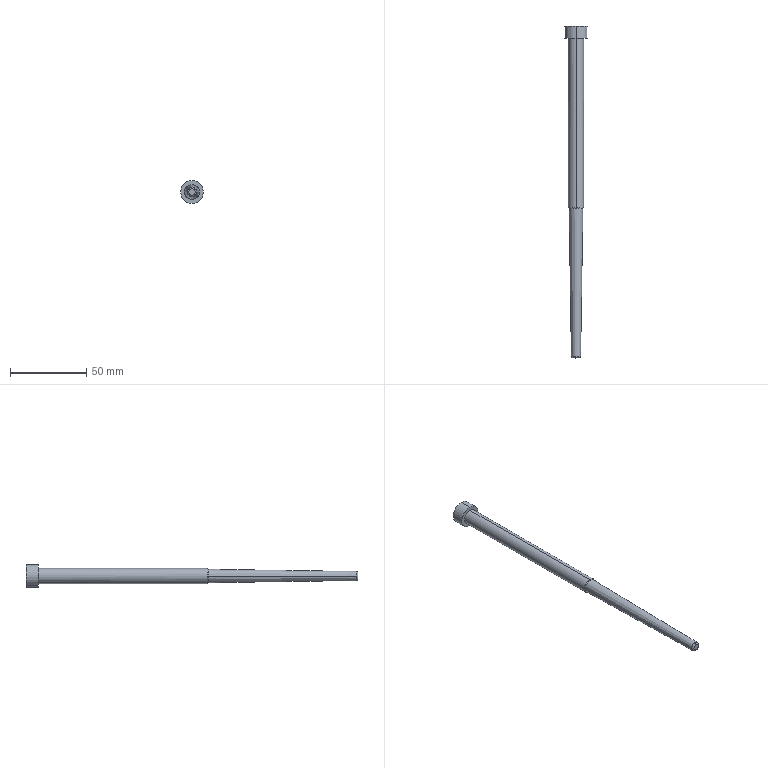Part | SolidWorks | features BaseBody 1 | 1 solid | 13 faces | box 15 x 218.233 x 15 mm | volume 14645 mm3 | cone 4 | cylinder 4 | plane 3 | torus 2 | commonest cylinder face diameters 10 x2 15 x2
STEP:
#1=CARTESIAN_POINT('',(103.861,100.091,21.065));
#2=VERTEX_POINT('',#1);
#3=CARTESIAN_POINT('',(94.826,100.091,21.065));
#4=VERTEX_POINT('',#3);
#5=CARTESIAN_POINT('',(99.343,100.091,21.065));
#6=DIRECTION('',(0.,1.,0.));
#7=DIRECTION('',(1.,0.,0.));
#8=AXIS2_PLACEMENT_3D('',#5,#6,#7);
#9=CIRCLE('',#8,4.517);
#10=EDGE_CURVE('',#2,#4,#9,.T.);
#11=ORIENTED_EDGE('',*,*,#10,.T.);
#12=CARTESIAN_POINT('',(94.343,100.567,21.065));
#13=VERTEX_POINT('',#12);
#14=CARTESIAN_POINT('',(94.826,100.091,21.065));
#15=DIRECTION('',(-0.7125,0.7017,0.));
#16=VECTOR('',#15,1000.);
#17=LINE('',#14,#16);
#18=EDGE_CURVE('',#4,#13,#17,.T.);
#19=ORIENTED_EDGE('',*,*,#18,.T.);
#20=CARTESIAN_POINT('',(99.343,100.567,16.065));
#21=VERTEX_POINT('',#20);
#22=CARTESIAN_POINT('',(99.343,100.567,21.065));
#23=DIRECTION('',(0.,1.,0.));
#24=DIRECTION('',(-1.,0.,0.));
#25=AXIS2_PLACEMENT_3D('',#22,#23,#24);
#26=CIRCLE('',#25,5.);
#27=EDGE_CURVE('',#21,#13,#26,.T.);
#28=ORIENTED_EDGE('',*,*,#27,.F.);
#29=CARTESIAN_POINT('',(104.343,100.567,21.065));
#30=VERTEX_POINT('',#29);
#31=CARTESIAN_POINT('',(99.343,100.567,21.065));
#32=DIRECTION('',(0.,1.,0.));
#33=DIRECTION('',(-1.,0.,0.));
#34=AXIS2_PLACEMENT_3D('',#31,#32,#33);
#35=CIRCLE('',#34,5.);
#36=EDGE_CURVE('',#30,#21,#35,.T.);
#37=ORIENTED_EDGE('',*,*,#36,.F.);
#38=CARTESIAN_POINT('',(103.861,100.091,21.065));
#39=DIRECTION('',(0.7125,0.7017,0.));
#40=VECTOR('',#39,1000.);
#41=LINE('',#38,#40);
#42=EDGE_CURVE('',#2,#30,#41,.T.);
#43=ORIENTED_EDGE('',*,*,#42,.F.);
#44=EDGE_LOOP('',(#11,#19,#28,#37,#43));
#45=FACE_OUTER_BOUND('',#44,.T.);
#46=CARTESIAN_POINT('',(99.343,100.091,21.065));
#47=DIRECTION('',(0.,1.,0.));
#48=DIRECTION('',(1.,0.,0.));
#49=AXIS2_PLACEMENT_3D('',#46,#47,#48);
#50=CONICAL_SURFACE('',#49,4.517,0.793);
#51=ADVANCED_FACE('',(#45),#50,.T.);
#52=CARTESIAN_POINT('',(96.304,2.757,21.065));
#53=VERTEX_POINT('',#52);
#54=CARTESIAN_POINT('',(99.343,2.757,18.026));
#55=VERTEX_POINT('',#54);
#56=CARTESIAN_POINT('',(99.343,2.757,21.065));
#57=DIRECTION('',(0.,-1.,0.));
#58=DIRECTION('',(0.,0.,-1.));
#59=AXIS2_PLACEMENT_3D('',#56,#57,#58);
#60=CIRCLE('',#59,3.039);
#61=EDGE_CURVE('',#53,#55,#60,.T.);
#62=ORIENTED_EDGE('',*,*,#61,.F.);
#63=CARTESIAN_POINT('',(94.819,100.594,21.065));
#64=DIRECTION('',(-0.01518,0.9999,0.));
#65=VECTOR('',#64,1000.);
#66=LINE('',#63,#65);
#67=EDGE_CURVE('',#53,#4,#66,.T.);
#68=ORIENTED_EDGE('',*,*,#67,.T.);
#69=ORIENTED_EDGE('',*,*,#10,.F.);
#70=CARTESIAN_POINT('',(102.382,2.757,21.065));
#71=VERTEX_POINT('',#70);
#72=CARTESIAN_POINT('',(103.868,100.594,21.065));
#73=DIRECTION('',(0.01518,0.9999,0.));
#74=VECTOR('',#73,1000.);
#75=LINE('',#72,#74);
#76=EDGE_CURVE('',#71,#2,#75,.T.);
#77=ORIENTED_EDGE('',*,*,#76,.F.);
#78=CARTESIAN_POINT('',(99.343,2.757,21.065));
#79=DIRECTION('',(0.,-1.,0.));
#80=DIRECTION('',(0.,0.,-1.));
#81=AXIS2_PLACEMENT_3D('',#78,#79,#80);
#82=CIRCLE('',#81,3.039);
#83=EDGE_CURVE('',#55,#71,#82,.T.);
#84=ORIENTED_EDGE('',*,*,#83,.F.);
#85=EDGE_LOOP('',(#62,#68,#69,#77,#84));
#86=FACE_OUTER_BOUND('',#85,.T.);
#87=CARTESIAN_POINT('',(99.343,100.594,21.065));
#88=DIRECTION('',(0.,1.,0.));
#89=DIRECTION('',(1.,0.,0.));
#90=AXIS2_PLACEMENT_3D('',#87,#88,#89);
#91=CONICAL_SURFACE('',#90,4.525,0.01518);
#92=ADVANCED_FACE('',(#86),#91,.T.);
#93=CARTESIAN_POINT('',(99.343,1.767,23.099));
#94=VERTEX_POINT('',#93);
#95=CARTESIAN_POINT('',(99.343,1.767,19.032));
#96=VERTEX_POINT('',#95);
#97=CARTESIAN_POINT('',(99.343,1.767,21.065));
#98=DIRECTION('',(0.,1.,0.));
#99=DIRECTION('',(0.,0.,1.));
#100=AXIS2_PLACEMENT_3D('',#97,#98,#99);
#101=CIRCLE('',#100,2.034);
#102=EDGE_CURVE('',#94,#96,#101,.T.);
#103=ORIENTED_EDGE('',*,*,#102,.T.);
#104=CARTESIAN_POINT('',(99.343,2.772,19.032));
#105=DIRECTION('',(1.,0.,0.));
#106=DIRECTION('',(0.,0.,-1.));
#107=AXIS2_PLACEMENT_3D('',#104,#105,#106);
#108=CIRCLE('',#107,1.005);
#109=EDGE_CURVE('',#96,#55,#108,.T.);
#110=ORIENTED_EDGE('',*,*,#109,.T.);
#111=ORIENTED_EDGE('',*,*,#83,.T.);
#112=CARTESIAN_POINT('',(99.343,2.757,24.104));
#113=VERTEX_POINT('',#112);
#114=CARTESIAN_POINT('',(99.343,2.757,21.065));
#115=DIRECTION('',(0.,-1.,0.));
#116=DIRECTION('',(0.,0.,-1.));
#117=AXIS2_PLACEMENT_3D('',#114,#115,#116);
#118=CIRCLE('',#117,3.039);
#119=EDGE_CURVE('',#71,#113,#118,.T.);
#120=ORIENTED_EDGE('',*,*,#119,.T.);
#121=CARTESIAN_POINT('',(99.343,2.772,23.099));
#122=DIRECTION('',(-1.,0.,0.));
#123=DIRECTION('',(0.,0.,1.));
#124=AXIS2_PLACEMENT_3D('',#121,#122,#123);
#125=CIRCLE('',#124,1.005);
#126=EDGE_CURVE('',#94,#113,#125,.T.);
#127=ORIENTED_EDGE('',*,*,#126,.F.);
#128=EDGE_LOOP('',(#103,#110,#111,#120,#127));
#129=FACE_OUTER_BOUND('',#128,.T.);
#130=CARTESIAN_POINT('',(99.343,2.772,21.065));
#131=DIRECTION('',(0.,1.,0.));
#132=DIRECTION('',(0.,0.,1.));
#133=AXIS2_PLACEMENT_3D('',#130,#131,#132);
#134=TOROIDAL_SURFACE('',#133,2.034,1.006);
#135=ADVANCED_FACE('',(#129),#134,.T.);
#136=CARTESIAN_POINT('',(99.343,220.,13.565));
#137=VERTEX_POINT('',#136);
#138=CARTESIAN_POINT('',(99.343,220.,28.565));
#139=VERTEX_POINT('',#138);
#140=CARTESIAN_POINT('',(99.343,220.,21.065));
#141=DIRECTION('',(0.,-1.,0.));
#142=DIRECTION('',(0.,0.,-1.));
#143=AXIS2_PLACEMENT_3D('',#140,#141,#142);
#144=CIRCLE('',#143,7.5);
#145=EDGE_CURVE('',#137,#139,#144,.T.);
#146=ORIENTED_EDGE('',*,*,#145,.T.);
#147=CARTESIAN_POINT('',(99.343,212.,28.565));
#148=VERTEX_POINT('',#147);
#149=CARTESIAN_POINT('',(99.343,220.,28.565));
#150=DIRECTION('',(0.,-1.,0.));
#151=VECTOR('',#150,1000.);
#152=LINE('',#149,#151);
#153=EDGE_CURVE('',#139,#148,#152,.T.);
#154=ORIENTED_EDGE('',*,*,#153,.T.);
#155=CARTESIAN_POINT('',(99.343,212.,13.565));
#156=VERTEX_POINT('',#155);
#157=CARTESIAN_POINT('',(99.343,212.,21.065));
#158=DIRECTION('',(0.,-1.,0.));
#159=DIRECTION('',(0.,0.,-1.));
#160=AXIS2_PLACEMENT_3D('',#157,#158,#159);
#161=CIRCLE('',#160,7.5);
#162=EDGE_CURVE('',#156,#148,#161,.T.);
#163=ORIENTED_EDGE('',*,*,#162,.F.);
#164=CARTESIAN_POINT('',(99.343,220.,13.565));
#165=DIRECTION('',(0.,-1.,0.));
#166=VECTOR('',#165,1000.);
#167=LINE('',#164,#166);
#168=EDGE_CURVE('',#137,#156,#167,.T.);
#169=ORIENTED_EDGE('',*,*,#168,.F.);
#170=EDGE_LOOP('',(#146,#154,#163,#169));
#171=FACE_OUTER_BOUND('',#170,.T.);
#172=CARTESIAN_POINT('',(99.343,220.,21.065));
#173=DIRECTION('',(0.,-1.,0.));
#174=DIRECTION('',(0.,0.,-1.));
#175=AXIS2_PLACEMENT_3D('',#172,#173,#174);
#176=CYLINDRICAL_SURFACE('',#175,7.5);
#177=ADVANCED_FACE('',(#171),#176,.T.);
#178=CARTESIAN_POINT('',(99.343,212.,26.065));
#179=VERTEX_POINT('',#178);
#180=CARTESIAN_POINT('',(99.343,212.,16.065));
#181=VERTEX_POINT('',#180);
#182=CARTESIAN_POINT('',(99.343,212.,21.065));
#183=DIRECTION('',(0.,1.,0.));
#184=DIRECTION('',(0.,0.,-1.));
#185=AXIS2_PLACEMENT_3D('',#182,#183,#184);
#186=CIRCLE('',#185,5.);
#187=EDGE_CURVE('',#179,#181,#186,.T.);
#188=ORIENTED_EDGE('',*,*,#187,.F.);
#189=CARTESIAN_POINT('',(99.343,100.567,26.065));
#190=VERTEX_POINT('',#189);
#191=CARTESIAN_POINT('',(99.343,100.594,26.065));
#192=DIRECTION('',(0.,-1.,0.));
#193=VECTOR('',#192,1000.);
#194=LINE('',#191,#193);
#195=EDGE_CURVE('',#179,#190,#194,.T.);
#196=ORIENTED_EDGE('',*,*,#195,.T.);
#197=CARTESIAN_POINT('',(99.343,100.567,21.065));
#198=DIRECTION('',(0.,1.,0.));
#199=DIRECTION('',(-1.,0.,0.));
#200=AXIS2_PLACEMENT_3D('',#197,#198,#199);
#201=CIRCLE('',#200,5.);
#202=EDGE_CURVE('',#190,#30,#201,.T.);
#203=ORIENTED_EDGE('',*,*,#202,.T.);
#204=ORIENTED_EDGE('',*,*,#36,.T.);
#205=CARTESIAN_POINT('',(99.343,100.594,16.065));
#206=DIRECTION('',(0.,-1.,0.));
#207=VECTOR('',#206,1000.);
#208=LINE('',#205,#207);
#209=EDGE_CURVE('',#181,#21,#208,.T.);
#210=ORIENTED_EDGE('',*,*,#209,.F.);
#211=EDGE_LOOP('',(#188,#196,#203,#204,#210));
#212=FACE_OUTER_BOUND('',#211,.T.);
#213=CARTESIAN_POINT('',(99.343,100.594,21.065));
#214=DIRECTION('',(0.,-1.,0.));
#215=DIRECTION('',(0.,0.,-1.));
#216=AXIS2_PLACEMENT_3D('',#213,#214,#215);
#217=CYLINDRICAL_SURFACE('',#216,5.);
#218=ADVANCED_FACE('',(#212),#217,.T.);
#219=ORIENTED_EDGE('',*,*,#195,.F.);
#220=CARTESIAN_POINT('',(99.343,212.,21.065));
#221=DIRECTION('',(0.,1.,0.));
#222=DIRECTION('',(0.,0.,-1.));
#223=AXIS2_PLACEMENT_3D('',#220,#221,#222);
#224=CIRCLE('',#223,5.);
#225=EDGE_CURVE('',#181,#179,#224,.T.);
#226=ORIENTED_EDGE('',*,*,#225,.F.);
#227=ORIENTED_EDGE('',*,*,#209,.T.);
#228=ORIENTED_EDGE('',*,*,#27,.T.);
#229=CARTESIAN_POINT('',(99.343,100.567,21.065));
#230=DIRECTION('',(0.,1.,0.));
#231=DIRECTION('',(-1.,0.,0.));
#232=AXIS2_PLACEMENT_3D('',#229,#230,#231);
#233=CIRCLE('',#232,5.);
#234=EDGE_CURVE('',#13,#190,#233,.T.);
#235=ORIENTED_EDGE('',*,*,#234,.T.);
#236=EDGE_LOOP('',(#219,#226,#227,#228,#235));
#237=FACE_OUTER_BOUND('',#236,.T.);
#238=CARTESIAN_POINT('',(99.343,100.594,21.065));
#239=DIRECTION('',(0.,-1.,0.));
#240=DIRECTION('',(0.,0.,-1.));
#241=AXIS2_PLACEMENT_3D('',#238,#239,#240);
#242=CYLINDRICAL_SURFACE('',#241,5.);
#243=ADVANCED_FACE('',(#237),#242,.T.);
#244=ORIENTED_EDGE('',*,*,#225,.T.);
#245=ORIENTED_EDGE('',*,*,#187,.T.);
#246=EDGE_LOOP('',(#244,#245));
#247=FACE_BOUND('',#246,.T.);
#248=ORIENTED_EDGE('',*,*,#162,.T.);
#249=CARTESIAN_POINT('',(99.343,212.,21.065));
#250=DIRECTION('',(0.,-1.,0.));
#251=DIRECTION('',(0.,0.,-1.));
#252=AXIS2_PLACEMENT_3D('',#249,#250,#251);
#253=CIRCLE('',#252,7.5);
#254=EDGE_CURVE('',#148,#156,#253,.T.);
#255=ORIENTED_EDGE('',*,*,#254,.T.);
#256=EDGE_LOOP('',(#248,#255));
#257=FACE_OUTER_BOUND('',#256,.T.);
#258=CARTESIAN_POINT('',(99.343,212.,21.065));
#259=DIRECTION('',(0.,-1.,0.));
#260=DIRECTION('',(0.,0.,-1.));
#261=AXIS2_PLACEMENT_3D('',#258,#259,#260);
#262=PLANE('',#261);
#263=ADVANCED_FACE('',(#247,#257),#262,.T.);
#264=ORIENTED_EDGE('',*,*,#153,.F.);
#265=CARTESIAN_POINT('',(99.343,220.,21.065));
#266=DIRECTION('',(0.,-1.,0.));
#267=DIRECTION('',(0.,0.,-1.));
#268=AXIS2_PLACEMENT_3D('',#265,#266,#267);
#269=CIRCLE('',#268,7.5);
#270=EDGE_CURVE('',#139,#137,#269,.T.);
#271=ORIENTED_EDGE('',*,*,#270,.T.);
#272=ORIENTED_EDGE('',*,*,#168,.T.);
#273=ORIENTED_EDGE('',*,*,#254,.F.);
#274=EDGE_LOOP('',(#264,#271,#272,#273));
#275=FACE_OUTER_BOUND('',#274,.T.);
#276=CARTESIAN_POINT('',(99.343,220.,21.065));
#277=DIRECTION('',(0.,-1.,0.));
#278=DIRECTION('',(0.,0.,-1.));
#279=AXIS2_PLACEMENT_3D('',#276,#277,#278);
#280=CYLINDRICAL_SURFACE('',#279,7.5);
#281=ADVANCED_FACE('',(#275),#280,.T.);
#282=ORIENTED_EDGE('',*,*,#102,.F.);
#283=CARTESIAN_POINT('',(99.343,1.767,21.065));
#284=DIRECTION('',(0.,1.,0.));
#285=DIRECTION('',(0.,0.,1.));
#286=AXIS2_PLACEMENT_3D('',#283,#284,#285);
#287=CIRCLE('',#286,2.034);
#288=EDGE_CURVE('',#96,#94,#287,.T.);
#289=ORIENTED_EDGE('',*,*,#288,.F.);
#290=EDGE_LOOP('',(#282,#289));
#291=FACE_OUTER_BOUND('',#290,.T.);
#292=CARTESIAN_POINT('',(107.137,1.767,25.251));
#293=DIRECTION('',(0.,1.,0.));
#294=DIRECTION('',(0.,0.,1.));
#295=AXIS2_PLACEMENT_3D('',#292,#293,#294);
#296=PLANE('',#295);
#297=ADVANCED_FACE('',(#291),#296,.F.);
#298=ORIENTED_EDGE('',*,*,#109,.F.);
#299=ORIENTED_EDGE('',*,*,#288,.T.);
#300=ORIENTED_EDGE('',*,*,#126,.T.);
#301=CARTESIAN_POINT('',(99.343,2.757,21.065));
#302=DIRECTION('',(0.,-1.,0.));
#303=DIRECTION('',(0.,0.,-1.));
#304=AXIS2_PLACEMENT_3D('',#301,#302,#303);
#305=CIRCLE('',#304,3.039);
#306=EDGE_CURVE('',#113,#53,#305,.T.);
#307=ORIENTED_EDGE('',*,*,#306,.T.);
#308=ORIENTED_EDGE('',*,*,#61,.T.);
#309=EDGE_LOOP('',(#298,#299,#300,#307,#308));
#310=FACE_OUTER_BOUND('',#309,.T.);
#311=CARTESIAN_POINT('',(99.343,2.772,21.065));
#312=DIRECTION('',(0.,1.,0.));
#313=DIRECTION('',(0.,0.,1.));
#314=AXIS2_PLACEMENT_3D('',#311,#312,#313);
#315=TOROIDAL_SURFACE('',#314,2.034,1.006);
#316=ADVANCED_FACE('',(#310),#315,.T.);
#317=ORIENTED_EDGE('',*,*,#67,.F.);
#318=ORIENTED_EDGE('',*,*,#306,.F.);
#319=ORIENTED_EDGE('',*,*,#119,.F.);
#320=ORIENTED_EDGE('',*,*,#76,.T.);
#321=CARTESIAN_POINT('',(99.343,100.091,21.065));
#322=DIRECTION('',(0.,1.,0.));
#323=DIRECTION('',(1.,0.,0.));
#324=AXIS2_PLACEMENT_3D('',#321,#322,#323);
#325=CIRCLE('',#324,4.517);
#326=EDGE_CURVE('',#4,#2,#325,.T.);
#327=ORIENTED_EDGE('',*,*,#326,.F.);
#328=EDGE_LOOP('',(#317,#318,#319,#320,#327));
#329=FACE_OUTER_BOUND('',#328,.T.);
#330=CARTESIAN_POINT('',(99.343,100.594,21.065));
#331=DIRECTION('',(0.,1.,0.));
#332=DIRECTION('',(1.,0.,0.));
#333=AXIS2_PLACEMENT_3D('',#330,#331,#332);
#334=CONICAL_SURFACE('',#333,4.525,0.01518);
#335=ADVANCED_FACE('',(#329),#334,.T.);
#336=ORIENTED_EDGE('',*,*,#18,.F.);
#337=ORIENTED_EDGE('',*,*,#326,.T.);
#338=ORIENTED_EDGE('',*,*,#42,.T.);
#339=ORIENTED_EDGE('',*,*,#202,.F.);
#340=ORIENTED_EDGE('',*,*,#234,.F.);
#341=EDGE_LOOP('',(#336,#337,#338,#339,#340));
#342=FACE_OUTER_BOUND('',#341,.T.);
#343=CARTESIAN_POINT('',(99.343,100.091,21.065));
#344=DIRECTION('',(0.,1.,0.));
#345=DIRECTION('',(1.,0.,0.));
#346=AXIS2_PLACEMENT_3D('',#343,#344,#345);
#347=CONICAL_SURFACE('',#346,4.517,0.793);
#348=ADVANCED_FACE('',(#342),#347,.T.);
#349=ORIENTED_EDGE('',*,*,#145,.F.);
#350=ORIENTED_EDGE('',*,*,#270,.F.);
#351=EDGE_LOOP('',(#349,#350));
#352=FACE_OUTER_BOUND('',#351,.T.);
#353=CARTESIAN_POINT('',(82.5,220.,5.));
#354=DIRECTION('',(0.,1.,0.));
#355=DIRECTION('',(0.,0.,1.));
#356=AXIS2_PLACEMENT_3D('',#353,#354,#355);
#357=PLANE('',#356);
#358=ADVANCED_FACE('',(#352),#357,.T.);
#359=CLOSED_SHELL('',(#51,#92,#135,#177,#218,#243,#263,#281,#297,#316,#335,#348,#358));
#360=MANIFOLD_SOLID_BREP('',#359);
#361=CARTESIAN_POINT('',(0.,0.,0.));
#362=DIRECTION('',(0.,0.,1.));
#363=DIRECTION('',(1.,0.,0.));
#364=AXIS2_PLACEMENT_3D('',#361,#362,#363);
#365=(LENGTH_UNIT()NAMED_UNIT(*)SI_UNIT(.MILLI.,.METRE.));
#366=UNCERTAINTY_MEASURE_WITH_UNIT(LENGTH_MEASURE(0.00001),#365,'','');
#367=(NAMED_UNIT(*)PLANE_ANGLE_UNIT()SI_UNIT($,.RADIAN.));
#368=(NAMED_UNIT(*)SI_UNIT($,.STERADIAN.)SOLID_ANGLE_UNIT());
#369=(GEOMETRIC_REPRESENTATION_CONTEXT(3)GLOBAL_UNCERTAINTY_ASSIGNED_CONTEXT((#366))GLOBAL_UNIT_ASSIGNED_CONTEXT((#365,#367,#368))REPRESENTATION_CONTEXT('',''));
#370=ADVANCED_BREP_SHAPE_REPRESENTATION('',(#360,#364),#369);